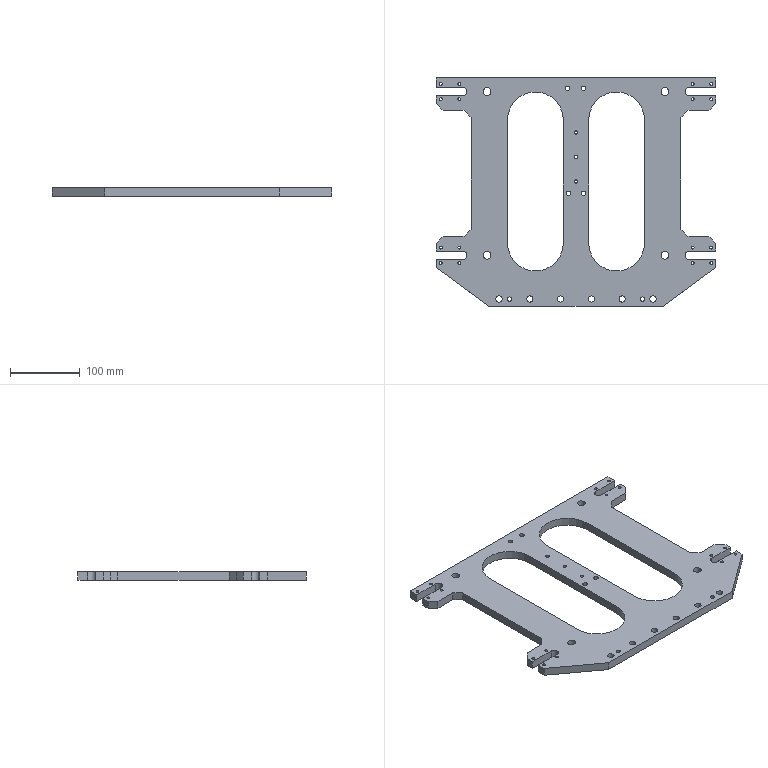Part | 1 solid | 83 faces | box 400 x 326 x 12 mm | volume 801311 mm3 | cylinder 43 | plane 40 | commonest cylinder face diameters 4.2 x16 9 x6 6.6 x4 11 x4 12 x4 80 x4